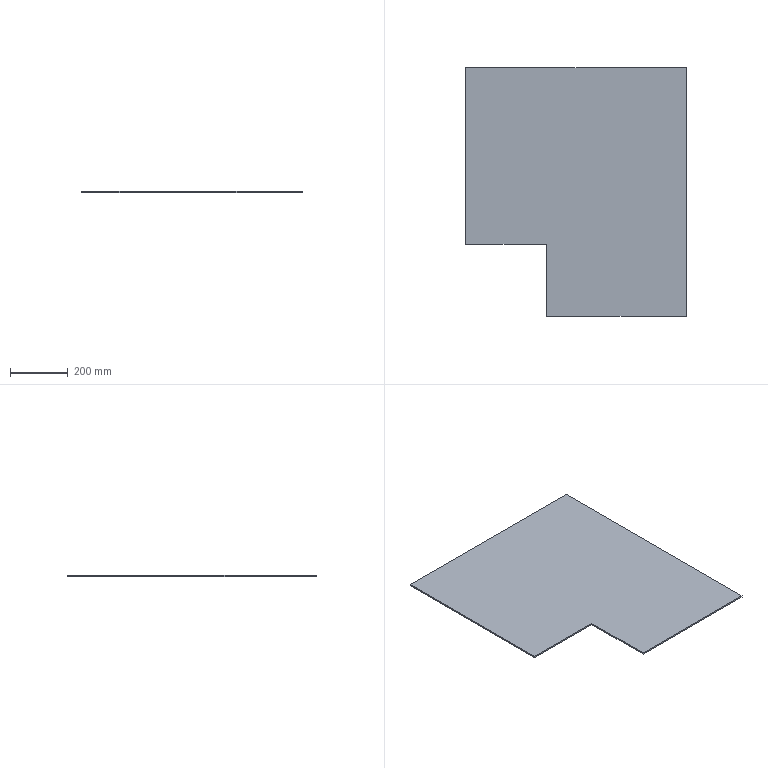Part | SolidWorks | features Extrusion 1, ICE 1 | 1 solid | 8 faces | box 764 x 860 x 5 mm | volume 2935200 mm3 | plane 8
STEP:
#1=CARTESIAN_POINT('',(-382.,430.,0.));
#2=VERTEX_POINT('',#1);
#3=CARTESIAN_POINT('',(-382.,-180.,0.));
#4=VERTEX_POINT('',#3);
#5=CARTESIAN_POINT('',(-382.,-430.,0.));
#6=DIRECTION('',(0.,-1.,0.));
#7=VECTOR('',#6,1000.);
#8=LINE('',#5,#7);
#9=EDGE_CURVE('',#2,#4,#8,.T.);
#10=ORIENTED_EDGE('',*,*,#9,.T.);
#11=CARTESIAN_POINT('',(-382.,-180.,5.));
#12=VERTEX_POINT('',#11);
#13=CARTESIAN_POINT('',(-382.,-180.,-0.001));
#14=DIRECTION('',(0.,0.,1.));
#15=VECTOR('',#14,1000.);
#16=LINE('',#13,#15);
#17=EDGE_CURVE('',#4,#12,#16,.T.);
#18=ORIENTED_EDGE('',*,*,#17,.T.);
#19=CARTESIAN_POINT('',(-382.,430.,5.));
#20=VERTEX_POINT('',#19);
#21=CARTESIAN_POINT('',(-382.,-430.,5.));
#22=DIRECTION('',(0.,-1.,0.));
#23=VECTOR('',#22,1000.);
#24=LINE('',#21,#23);
#25=EDGE_CURVE('',#20,#12,#24,.T.);
#26=ORIENTED_EDGE('',*,*,#25,.F.);
#27=CARTESIAN_POINT('',(-382.,430.,5.));
#28=DIRECTION('',(0.,0.,-1.));
#29=VECTOR('',#28,1000.);
#30=LINE('',#27,#29);
#31=EDGE_CURVE('',#20,#2,#30,.T.);
#32=ORIENTED_EDGE('',*,*,#31,.T.);
#33=EDGE_LOOP('',(#10,#18,#26,#32));
#34=FACE_OUTER_BOUND('',#33,.T.);
#35=CARTESIAN_POINT('',(-382.,-430.,5.));
#36=DIRECTION('',(1.,0.,0.));
#37=DIRECTION('',(0.,0.,-1.));
#38=AXIS2_PLACEMENT_3D('',#35,#36,#37);
#39=PLANE('',#38);
#40=ADVANCED_FACE('',(#34),#39,.F.);
#41=CARTESIAN_POINT('',(-102.,-430.,5.));
#42=VERTEX_POINT('',#41);
#43=CARTESIAN_POINT('',(382.,-430.,5.));
#44=VERTEX_POINT('',#43);
#45=CARTESIAN_POINT('',(382.,-430.,5.));
#46=DIRECTION('',(1.,0.,0.));
#47=VECTOR('',#46,1000.);
#48=LINE('',#45,#47);
#49=EDGE_CURVE('',#42,#44,#48,.T.);
#50=ORIENTED_EDGE('',*,*,#49,.F.);
#51=CARTESIAN_POINT('',(-102.,-430.,0.));
#52=VERTEX_POINT('',#51);
#53=CARTESIAN_POINT('',(-102.,-430.,-0.001));
#54=DIRECTION('',(0.,0.,1.));
#55=VECTOR('',#54,1000.);
#56=LINE('',#53,#55);
#57=EDGE_CURVE('',#52,#42,#56,.T.);
#58=ORIENTED_EDGE('',*,*,#57,.F.);
#59=CARTESIAN_POINT('',(382.,-430.,0.));
#60=VERTEX_POINT('',#59);
#61=CARTESIAN_POINT('',(382.,-430.,0.));
#62=DIRECTION('',(1.,0.,0.));
#63=VECTOR('',#62,1000.);
#64=LINE('',#61,#63);
#65=EDGE_CURVE('',#52,#60,#64,.T.);
#66=ORIENTED_EDGE('',*,*,#65,.T.);
#67=CARTESIAN_POINT('',(382.,-430.,5.));
#68=DIRECTION('',(0.,0.,-1.));
#69=VECTOR('',#68,1000.);
#70=LINE('',#67,#69);
#71=EDGE_CURVE('',#44,#60,#70,.T.);
#72=ORIENTED_EDGE('',*,*,#71,.F.);
#73=EDGE_LOOP('',(#50,#58,#66,#72));
#74=FACE_OUTER_BOUND('',#73,.T.);
#75=CARTESIAN_POINT('',(382.,-430.,5.));
#76=DIRECTION('',(0.,1.,0.));
#77=DIRECTION('',(-1.,0.,0.));
#78=AXIS2_PLACEMENT_3D('',#75,#76,#77);
#79=PLANE('',#78);
#80=ADVANCED_FACE('',(#74),#79,.F.);
#81=CARTESIAN_POINT('',(382.,430.,0.));
#82=VERTEX_POINT('',#81);
#83=CARTESIAN_POINT('',(382.,-430.,0.));
#84=DIRECTION('',(0.,1.,0.));
#85=VECTOR('',#84,1000.);
#86=LINE('',#83,#85);
#87=EDGE_CURVE('',#60,#82,#86,.T.);
#88=ORIENTED_EDGE('',*,*,#87,.T.);
#89=CARTESIAN_POINT('',(382.,430.,5.));
#90=VERTEX_POINT('',#89);
#91=CARTESIAN_POINT('',(382.,430.,5.));
#92=DIRECTION('',(0.,0.,-1.));
#93=VECTOR('',#92,1000.);
#94=LINE('',#91,#93);
#95=EDGE_CURVE('',#90,#82,#94,.T.);
#96=ORIENTED_EDGE('',*,*,#95,.F.);
#97=CARTESIAN_POINT('',(382.,-430.,5.));
#98=DIRECTION('',(0.,1.,0.));
#99=VECTOR('',#98,1000.);
#100=LINE('',#97,#99);
#101=EDGE_CURVE('',#44,#90,#100,.T.);
#102=ORIENTED_EDGE('',*,*,#101,.F.);
#103=ORIENTED_EDGE('',*,*,#71,.T.);
#104=EDGE_LOOP('',(#88,#96,#102,#103));
#105=FACE_OUTER_BOUND('',#104,.T.);
#106=CARTESIAN_POINT('',(382.,-430.,5.));
#107=DIRECTION('',(-1.,0.,0.));
#108=DIRECTION('',(0.,0.,1.));
#109=AXIS2_PLACEMENT_3D('',#106,#107,#108);
#110=PLANE('',#109);
#111=ADVANCED_FACE('',(#105),#110,.F.);
#112=CARTESIAN_POINT('',(382.,430.,0.));
#113=DIRECTION('',(-1.,0.,0.));
#114=VECTOR('',#113,1000.);
#115=LINE('',#112,#114);
#116=EDGE_CURVE('',#82,#2,#115,.T.);
#117=ORIENTED_EDGE('',*,*,#116,.T.);
#118=ORIENTED_EDGE('',*,*,#31,.F.);
#119=CARTESIAN_POINT('',(382.,430.,5.));
#120=DIRECTION('',(-1.,0.,0.));
#121=VECTOR('',#120,1000.);
#122=LINE('',#119,#121);
#123=EDGE_CURVE('',#90,#20,#122,.T.);
#124=ORIENTED_EDGE('',*,*,#123,.F.);
#125=ORIENTED_EDGE('',*,*,#95,.T.);
#126=EDGE_LOOP('',(#117,#118,#124,#125));
#127=FACE_OUTER_BOUND('',#126,.T.);
#128=CARTESIAN_POINT('',(382.,430.,5.));
#129=DIRECTION('',(0.,-1.,0.));
#130=DIRECTION('',(1.,0.,0.));
#131=AXIS2_PLACEMENT_3D('',#128,#129,#130);
#132=PLANE('',#131);
#133=ADVANCED_FACE('',(#127),#132,.F.);
#134=CARTESIAN_POINT('',(-102.,-180.,5.));
#135=VERTEX_POINT('',#134);
#136=CARTESIAN_POINT('',(-382.,-180.,5.));
#137=DIRECTION('',(-1.,0.,0.));
#138=VECTOR('',#137,1000.);
#139=LINE('',#136,#138);
#140=EDGE_CURVE('',#135,#12,#139,.T.);
#141=ORIENTED_EDGE('',*,*,#140,.F.);
#142=CARTESIAN_POINT('',(-102.,-430.,5.));
#143=DIRECTION('',(0.,1.,0.));
#144=VECTOR('',#143,1000.);
#145=LINE('',#142,#144);
#146=EDGE_CURVE('',#42,#135,#145,.T.);
#147=ORIENTED_EDGE('',*,*,#146,.F.);
#148=ORIENTED_EDGE('',*,*,#49,.T.);
#149=ORIENTED_EDGE('',*,*,#101,.T.);
#150=ORIENTED_EDGE('',*,*,#123,.T.);
#151=ORIENTED_EDGE('',*,*,#25,.T.);
#152=EDGE_LOOP('',(#141,#147,#148,#149,#150,#151));
#153=FACE_OUTER_BOUND('',#152,.T.);
#154=CARTESIAN_POINT('',(0.,0.,5.));
#155=DIRECTION('',(0.,0.,1.));
#156=DIRECTION('',(1.,0.,0.));
#157=AXIS2_PLACEMENT_3D('',#154,#155,#156);
#158=PLANE('',#157);
#159=ADVANCED_FACE('',(#153),#158,.T.);
#160=CARTESIAN_POINT('',(-102.,-180.,0.));
#161=VERTEX_POINT('',#160);
#162=CARTESIAN_POINT('',(-102.,-430.,0.));
#163=DIRECTION('',(0.,-1.,0.));
#164=VECTOR('',#163,1000.);
#165=LINE('',#162,#164);
#166=EDGE_CURVE('',#161,#52,#165,.T.);
#167=ORIENTED_EDGE('',*,*,#166,.F.);
#168=CARTESIAN_POINT('',(-382.,-180.,0.));
#169=DIRECTION('',(1.,0.,0.));
#170=VECTOR('',#169,1000.);
#171=LINE('',#168,#170);
#172=EDGE_CURVE('',#4,#161,#171,.T.);
#173=ORIENTED_EDGE('',*,*,#172,.F.);
#174=ORIENTED_EDGE('',*,*,#9,.F.);
#175=ORIENTED_EDGE('',*,*,#116,.F.);
#176=ORIENTED_EDGE('',*,*,#87,.F.);
#177=ORIENTED_EDGE('',*,*,#65,.F.);
#178=EDGE_LOOP('',(#167,#173,#174,#175,#176,#177));
#179=FACE_OUTER_BOUND('',#178,.T.);
#180=CARTESIAN_POINT('',(0.,0.,0.));
#181=DIRECTION('',(0.,0.,1.));
#182=DIRECTION('',(1.,0.,0.));
#183=AXIS2_PLACEMENT_3D('',#180,#181,#182);
#184=PLANE('',#183);
#185=ADVANCED_FACE('',(#179),#184,.F.);
#186=ORIENTED_EDGE('',*,*,#172,.T.);
#187=CARTESIAN_POINT('',(-102.,-180.,-0.001));
#188=DIRECTION('',(0.,0.,1.));
#189=VECTOR('',#188,1000.);
#190=LINE('',#187,#189);
#191=EDGE_CURVE('',#161,#135,#190,.T.);
#192=ORIENTED_EDGE('',*,*,#191,.T.);
#193=ORIENTED_EDGE('',*,*,#140,.T.);
#194=ORIENTED_EDGE('',*,*,#17,.F.);
#195=EDGE_LOOP('',(#186,#192,#193,#194));
#196=FACE_OUTER_BOUND('',#195,.T.);
#197=CARTESIAN_POINT('',(-382.,-180.,-0.001));
#198=DIRECTION('',(0.,1.,0.));
#199=DIRECTION('',(0.,0.,1.));
#200=AXIS2_PLACEMENT_3D('',#197,#198,#199);
#201=PLANE('',#200);
#202=ADVANCED_FACE('',(#196),#201,.F.);
#203=ORIENTED_EDGE('',*,*,#166,.T.);
#204=ORIENTED_EDGE('',*,*,#57,.T.);
#205=ORIENTED_EDGE('',*,*,#146,.T.);
#206=ORIENTED_EDGE('',*,*,#191,.F.);
#207=EDGE_LOOP('',(#203,#204,#205,#206));
#208=FACE_OUTER_BOUND('',#207,.T.);
#209=CARTESIAN_POINT('',(-102.,-430.,-0.001));
#210=DIRECTION('',(1.,0.,0.));
#211=DIRECTION('',(0.,0.,-1.));
#212=AXIS2_PLACEMENT_3D('',#209,#210,#211);
#213=PLANE('',#212);
#214=ADVANCED_FACE('',(#208),#213,.F.);
#215=CLOSED_SHELL('',(#40,#80,#111,#133,#159,#185,#202,#214));
#216=MANIFOLD_SOLID_BREP('',#215);
#217=CARTESIAN_POINT('',(0.,0.,0.));
#218=DIRECTION('',(0.,0.,1.));
#219=DIRECTION('',(1.,0.,0.));
#220=AXIS2_PLACEMENT_3D('',#217,#218,#219);
#221=(LENGTH_UNIT()NAMED_UNIT(*)SI_UNIT(.MILLI.,.METRE.));
#222=UNCERTAINTY_MEASURE_WITH_UNIT(LENGTH_MEASURE(0.00001),#221,'','');
#223=(NAMED_UNIT(*)PLANE_ANGLE_UNIT()SI_UNIT($,.RADIAN.));
#224=(NAMED_UNIT(*)SI_UNIT($,.STERADIAN.)SOLID_ANGLE_UNIT());
#225=(GEOMETRIC_REPRESENTATION_CONTEXT(3)GLOBAL_UNCERTAINTY_ASSIGNED_CONTEXT((#222))GLOBAL_UNIT_ASSIGNED_CONTEXT((#221,#223,#224))REPRESENTATION_CONTEXT('',''));
#226=ADVANCED_BREP_SHAPE_REPRESENTATION('',(#216,#220),#225);